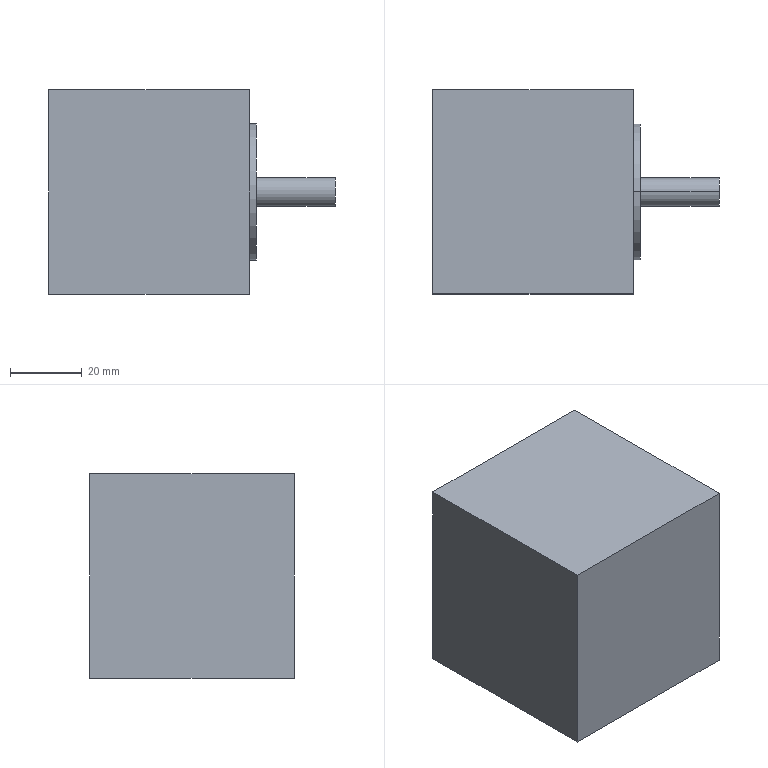Part | SolidWorks | features BaseBody 1 | 1 solid | 36 faces | box 80 x 57 x 57 mm | volume 184911 mm3 | cylinder 20 | plane 16 | commonest cylinder face diameters 3.4 x8 4.3 x8 8 x2 38 x2
STEP:
#1=CARTESIAN_POINT('',(-6.2,-23.57,25.72));
#2=VERTEX_POINT('',#1);
#3=CARTESIAN_POINT('',(-6.2,-23.57,21.42));
#4=VERTEX_POINT('',#3);
#5=CARTESIAN_POINT('',(-6.2,-23.57,23.57));
#6=DIRECTION('',(1.,0.,0.));
#7=DIRECTION('',(0.,0.,-1.));
#8=AXIS2_PLACEMENT_3D('',#5,#6,#7);
#9=CIRCLE('',#8,2.15);
#10=EDGE_CURVE('',#2,#4,#9,.T.);
#11=ORIENTED_EDGE('',*,*,#10,.F.);
#12=CARTESIAN_POINT('',(0.,-23.57,25.72));
#13=VERTEX_POINT('',#12);
#14=CARTESIAN_POINT('',(-6.2,-23.57,25.72));
#15=DIRECTION('',(1.,0.,0.));
#16=VECTOR('',#15,1000.);
#17=LINE('',#14,#16);
#18=EDGE_CURVE('',#2,#13,#17,.T.);
#19=ORIENTED_EDGE('',*,*,#18,.T.);
#20=CARTESIAN_POINT('',(0.,-23.57,21.42));
#21=VERTEX_POINT('',#20);
#22=CARTESIAN_POINT('',(0.,-23.57,23.57));
#23=DIRECTION('',(-1.,0.,0.));
#24=DIRECTION('',(0.,0.,-1.));
#25=AXIS2_PLACEMENT_3D('',#22,#23,#24);
#26=CIRCLE('',#25,2.15);
#27=EDGE_CURVE('',#21,#13,#26,.T.);
#28=ORIENTED_EDGE('',*,*,#27,.F.);
#29=CARTESIAN_POINT('',(-6.2,-23.57,21.42));
#30=DIRECTION('',(1.,0.,0.));
#31=VECTOR('',#30,1000.);
#32=LINE('',#29,#31);
#33=EDGE_CURVE('',#4,#21,#32,.T.);
#34=ORIENTED_EDGE('',*,*,#33,.F.);
#35=EDGE_LOOP('',(#11,#19,#28,#34));
#36=FACE_OUTER_BOUND('',#35,.T.);
#37=CARTESIAN_POINT('',(-6.2,-23.57,23.57));
#38=DIRECTION('',(1.,0.,0.));
#39=DIRECTION('',(0.,0.,-1.));
#40=AXIS2_PLACEMENT_3D('',#37,#38,#39);
#41=CYLINDRICAL_SURFACE('',#40,2.15);
#42=ADVANCED_FACE('',(#36),#41,.F.);
#43=CARTESIAN_POINT('',(-6.2,-23.57,-21.42));
#44=VERTEX_POINT('',#43);
#45=CARTESIAN_POINT('',(-6.2,-23.57,-25.72));
#46=VERTEX_POINT('',#45);
#47=CARTESIAN_POINT('',(-6.2,-23.57,-23.57));
#48=DIRECTION('',(1.,0.,0.));
#49=DIRECTION('',(0.,0.,-1.));
#50=AXIS2_PLACEMENT_3D('',#47,#48,#49);
#51=CIRCLE('',#50,2.15);
#52=EDGE_CURVE('',#44,#46,#51,.T.);
#53=ORIENTED_EDGE('',*,*,#52,.F.);
#54=CARTESIAN_POINT('',(0.,-23.57,-21.42));
#55=VERTEX_POINT('',#54);
#56=CARTESIAN_POINT('',(-6.2,-23.57,-21.42));
#57=DIRECTION('',(1.,0.,0.));
#58=VECTOR('',#57,1000.);
#59=LINE('',#56,#58);
#60=EDGE_CURVE('',#44,#55,#59,.T.);
#61=ORIENTED_EDGE('',*,*,#60,.T.);
#62=CARTESIAN_POINT('',(0.,-23.57,-25.72));
#63=VERTEX_POINT('',#62);
#64=CARTESIAN_POINT('',(0.,-23.57,-23.57));
#65=DIRECTION('',(-1.,0.,0.));
#66=DIRECTION('',(0.,0.,-1.));
#67=AXIS2_PLACEMENT_3D('',#64,#65,#66);
#68=CIRCLE('',#67,2.15);
#69=EDGE_CURVE('',#63,#55,#68,.T.);
#70=ORIENTED_EDGE('',*,*,#69,.F.);
#71=CARTESIAN_POINT('',(-6.2,-23.57,-25.72));
#72=DIRECTION('',(1.,0.,0.));
#73=VECTOR('',#72,1000.);
#74=LINE('',#71,#73);
#75=EDGE_CURVE('',#46,#63,#74,.T.);
#76=ORIENTED_EDGE('',*,*,#75,.F.);
#77=EDGE_LOOP('',(#53,#61,#70,#76));
#78=FACE_OUTER_BOUND('',#77,.T.);
#79=CARTESIAN_POINT('',(-6.2,-23.57,-23.57));
#80=DIRECTION('',(1.,0.,0.));
#81=DIRECTION('',(0.,0.,-1.));
#82=AXIS2_PLACEMENT_3D('',#79,#80,#81);
#83=CYLINDRICAL_SURFACE('',#82,2.15);
#84=ADVANCED_FACE('',(#78),#83,.F.);
#85=CARTESIAN_POINT('',(0.,0.,19.));
#86=VERTEX_POINT('',#85);
#87=CARTESIAN_POINT('',(0.,0.,-19.));
#88=VERTEX_POINT('',#87);
#89=CARTESIAN_POINT('',(0.,0.,0.));
#90=DIRECTION('',(-1.,0.,0.));
#91=DIRECTION('',(0.,0.,-1.));
#92=AXIS2_PLACEMENT_3D('',#89,#90,#91);
#93=CIRCLE('',#92,19.);
#94=EDGE_CURVE('',#86,#88,#93,.T.);
#95=ORIENTED_EDGE('',*,*,#94,.F.);
#96=CARTESIAN_POINT('',(2.,0.,19.));
#97=VERTEX_POINT('',#96);
#98=CARTESIAN_POINT('',(0.,0.,19.));
#99=DIRECTION('',(1.,0.,0.));
#100=VECTOR('',#99,1000.);
#101=LINE('',#98,#100);
#102=EDGE_CURVE('',#86,#97,#101,.T.);
#103=ORIENTED_EDGE('',*,*,#102,.T.);
#104=CARTESIAN_POINT('',(2.,0.,-19.));
#105=VERTEX_POINT('',#104);
#106=CARTESIAN_POINT('',(2.,0.,0.));
#107=DIRECTION('',(-1.,0.,0.));
#108=DIRECTION('',(0.,0.,-1.));
#109=AXIS2_PLACEMENT_3D('',#106,#107,#108);
#110=CIRCLE('',#109,19.);
#111=EDGE_CURVE('',#97,#105,#110,.T.);
#112=ORIENTED_EDGE('',*,*,#111,.T.);
#113=CARTESIAN_POINT('',(0.,0.,-19.));
#114=DIRECTION('',(1.,0.,0.));
#115=VECTOR('',#114,1000.);
#116=LINE('',#113,#115);
#117=EDGE_CURVE('',#88,#105,#116,.T.);
#118=ORIENTED_EDGE('',*,*,#117,.F.);
#119=EDGE_LOOP('',(#95,#103,#112,#118));
#120=FACE_OUTER_BOUND('',#119,.T.);
#121=CARTESIAN_POINT('',(0.,0.,0.));
#122=DIRECTION('',(1.,0.,0.));
#123=DIRECTION('',(0.,0.,-1.));
#124=AXIS2_PLACEMENT_3D('',#121,#122,#123);
#125=CYLINDRICAL_SURFACE('',#124,19.);
#126=ADVANCED_FACE('',(#120),#125,.T.);
#127=CARTESIAN_POINT('',(-6.2,23.57,25.72));
#128=VERTEX_POINT('',#127);
#129=CARTESIAN_POINT('',(-6.2,23.57,21.42));
#130=VERTEX_POINT('',#129);
#131=CARTESIAN_POINT('',(-6.2,23.57,23.57));
#132=DIRECTION('',(1.,0.,0.));
#133=DIRECTION('',(0.,0.,-1.));
#134=AXIS2_PLACEMENT_3D('',#131,#132,#133);
#135=CIRCLE('',#134,2.15);
#136=EDGE_CURVE('',#128,#130,#135,.T.);
#137=ORIENTED_EDGE('',*,*,#136,.F.);
#138=CARTESIAN_POINT('',(0.,23.57,25.72));
#139=VERTEX_POINT('',#138);
#140=CARTESIAN_POINT('',(-6.2,23.57,25.72));
#141=DIRECTION('',(1.,0.,0.));
#142=VECTOR('',#141,1000.);
#143=LINE('',#140,#142);
#144=EDGE_CURVE('',#128,#139,#143,.T.);
#145=ORIENTED_EDGE('',*,*,#144,.T.);
#146=CARTESIAN_POINT('',(0.,23.57,21.42));
#147=VERTEX_POINT('',#146);
#148=CARTESIAN_POINT('',(0.,23.57,23.57));
#149=DIRECTION('',(-1.,0.,0.));
#150=DIRECTION('',(0.,0.,-1.));
#151=AXIS2_PLACEMENT_3D('',#148,#149,#150);
#152=CIRCLE('',#151,2.15);
#153=EDGE_CURVE('',#147,#139,#152,.T.);
#154=ORIENTED_EDGE('',*,*,#153,.F.);
#155=CARTESIAN_POINT('',(-6.2,23.57,21.42));
#156=DIRECTION('',(1.,0.,0.));
#157=VECTOR('',#156,1000.);
#158=LINE('',#155,#157);
#159=EDGE_CURVE('',#130,#147,#158,.T.);
#160=ORIENTED_EDGE('',*,*,#159,.F.);
#161=EDGE_LOOP('',(#137,#145,#154,#160));
#162=FACE_OUTER_BOUND('',#161,.T.);
#163=CARTESIAN_POINT('',(-6.2,23.57,23.57));
#164=DIRECTION('',(1.,0.,0.));
#165=DIRECTION('',(0.,0.,-1.));
#166=AXIS2_PLACEMENT_3D('',#163,#164,#165);
#167=CYLINDRICAL_SURFACE('',#166,2.15);
#168=ADVANCED_FACE('',(#162),#167,.F.);
#169=CARTESIAN_POINT('',(-6.2,23.57,-21.42));
#170=VERTEX_POINT('',#169);
#171=CARTESIAN_POINT('',(-6.2,23.57,-25.72));
#172=VERTEX_POINT('',#171);
#173=CARTESIAN_POINT('',(-6.2,23.57,-23.57));
#174=DIRECTION('',(1.,0.,0.));
#175=DIRECTION('',(0.,0.,-1.));
#176=AXIS2_PLACEMENT_3D('',#173,#174,#175);
#177=CIRCLE('',#176,2.15);
#178=EDGE_CURVE('',#170,#172,#177,.T.);
#179=ORIENTED_EDGE('',*,*,#178,.F.);
#180=CARTESIAN_POINT('',(0.,23.57,-21.42));
#181=VERTEX_POINT('',#180);
#182=CARTESIAN_POINT('',(-6.2,23.57,-21.42));
#183=DIRECTION('',(1.,0.,0.));
#184=VECTOR('',#183,1000.);
#185=LINE('',#182,#184);
#186=EDGE_CURVE('',#170,#181,#185,.T.);
#187=ORIENTED_EDGE('',*,*,#186,.T.);
#188=CARTESIAN_POINT('',(0.,23.57,-25.72));
#189=VERTEX_POINT('',#188);
#190=CARTESIAN_POINT('',(0.,23.57,-23.57));
#191=DIRECTION('',(-1.,0.,0.));
#192=DIRECTION('',(0.,0.,-1.));
#193=AXIS2_PLACEMENT_3D('',#190,#191,#192);
#194=CIRCLE('',#193,2.15);
#195=EDGE_CURVE('',#189,#181,#194,.T.);
#196=ORIENTED_EDGE('',*,*,#195,.F.);
#197=CARTESIAN_POINT('',(-6.2,23.57,-25.72));
#198=DIRECTION('',(1.,0.,0.));
#199=VECTOR('',#198,1000.);
#200=LINE('',#197,#199);
#201=EDGE_CURVE('',#172,#189,#200,.T.);
#202=ORIENTED_EDGE('',*,*,#201,.F.);
#203=EDGE_LOOP('',(#179,#187,#196,#202));
#204=FACE_OUTER_BOUND('',#203,.T.);
#205=CARTESIAN_POINT('',(-6.2,23.57,-23.57));
#206=DIRECTION('',(1.,0.,0.));
#207=DIRECTION('',(0.,0.,-1.));
#208=AXIS2_PLACEMENT_3D('',#205,#206,#207);
#209=CYLINDRICAL_SURFACE('',#208,2.15);
#210=ADVANCED_FACE('',(#204),#209,.F.);
#211=CARTESIAN_POINT('',(-7.5,-23.57,25.27));
#212=VERTEX_POINT('',#211);
#213=CARTESIAN_POINT('',(-7.5,-23.57,21.87));
#214=VERTEX_POINT('',#213);
#215=CARTESIAN_POINT('',(-7.5,-23.57,23.57));
#216=DIRECTION('',(1.,0.,0.));
#217=DIRECTION('',(0.,0.,-1.));
#218=AXIS2_PLACEMENT_3D('',#215,#216,#217);
#219=CIRCLE('',#218,1.7);
#220=EDGE_CURVE('',#212,#214,#219,.T.);
#221=ORIENTED_EDGE('',*,*,#220,.F.);
#222=CARTESIAN_POINT('',(-6.2,-23.57,25.27));
#223=VERTEX_POINT('',#222);
#224=CARTESIAN_POINT('',(-7.5,-23.57,25.27));
#225=DIRECTION('',(1.,0.,0.));
#226=VECTOR('',#225,1000.);
#227=LINE('',#224,#226);
#228=EDGE_CURVE('',#212,#223,#227,.T.);
#229=ORIENTED_EDGE('',*,*,#228,.T.);
#230=CARTESIAN_POINT('',(-6.2,-23.57,21.87));
#231=VERTEX_POINT('',#230);
#232=CARTESIAN_POINT('',(-6.2,-23.57,23.57));
#233=DIRECTION('',(-1.,0.,0.));
#234=DIRECTION('',(0.,0.,-1.));
#235=AXIS2_PLACEMENT_3D('',#232,#233,#234);
#236=CIRCLE('',#235,1.7);
#237=EDGE_CURVE('',#231,#223,#236,.T.);
#238=ORIENTED_EDGE('',*,*,#237,.F.);
#239=CARTESIAN_POINT('',(-7.5,-23.57,21.87));
#240=DIRECTION('',(1.,0.,0.));
#241=VECTOR('',#240,1000.);
#242=LINE('',#239,#241);
#243=EDGE_CURVE('',#214,#231,#242,.T.);
#244=ORIENTED_EDGE('',*,*,#243,.F.);
#245=EDGE_LOOP('',(#221,#229,#238,#244));
#246=FACE_OUTER_BOUND('',#245,.T.);
#247=CARTESIAN_POINT('',(-7.5,-23.57,23.57));
#248=DIRECTION('',(1.,0.,0.));
#249=DIRECTION('',(0.,0.,-1.));
#250=AXIS2_PLACEMENT_3D('',#247,#248,#249);
#251=CYLINDRICAL_SURFACE('',#250,1.7);
#252=ADVANCED_FACE('',(#246),#251,.F.);
#253=CARTESIAN_POINT('',(-7.5,-23.57,-21.87));
#254=VERTEX_POINT('',#253);
#255=CARTESIAN_POINT('',(-7.5,-23.57,-25.27));
#256=VERTEX_POINT('',#255);
#257=CARTESIAN_POINT('',(-7.5,-23.57,-23.57));
#258=DIRECTION('',(1.,0.,0.));
#259=DIRECTION('',(0.,0.,-1.));
#260=AXIS2_PLACEMENT_3D('',#257,#258,#259);
#261=CIRCLE('',#260,1.7);
#262=EDGE_CURVE('',#254,#256,#261,.T.);
#263=ORIENTED_EDGE('',*,*,#262,.F.);
#264=CARTESIAN_POINT('',(-6.2,-23.57,-21.87));
#265=VERTEX_POINT('',#264);
#266=CARTESIAN_POINT('',(-7.5,-23.57,-21.87));
#267=DIRECTION('',(1.,0.,0.));
#268=VECTOR('',#267,1000.);
#269=LINE('',#266,#268);
#270=EDGE_CURVE('',#254,#265,#269,.T.);
#271=ORIENTED_EDGE('',*,*,#270,.T.);
#272=CARTESIAN_POINT('',(-6.2,-23.57,-25.27));
#273=VERTEX_POINT('',#272);
#274=CARTESIAN_POINT('',(-6.2,-23.57,-23.57));
#275=DIRECTION('',(-1.,0.,0.));
#276=DIRECTION('',(0.,0.,-1.));
#277=AXIS2_PLACEMENT_3D('',#274,#275,#276);
#278=CIRCLE('',#277,1.7);
#279=EDGE_CURVE('',#273,#265,#278,.T.);
#280=ORIENTED_EDGE('',*,*,#279,.F.);
#281=CARTESIAN_POINT('',(-7.5,-23.57,-25.27));
#282=DIRECTION('',(1.,0.,0.));
#283=VECTOR('',#282,1000.);
#284=LINE('',#281,#283);
#285=EDGE_CURVE('',#256,#273,#284,.T.);
#286=ORIENTED_EDGE('',*,*,#285,.F.);
#287=EDGE_LOOP('',(#263,#271,#280,#286));
#288=FACE_OUTER_BOUND('',#287,.T.);
#289=CARTESIAN_POINT('',(-7.5,-23.57,-23.57));
#290=DIRECTION('',(1.,0.,0.));
#291=DIRECTION('',(0.,0.,-1.));
#292=AXIS2_PLACEMENT_3D('',#289,#290,#291);
#293=CYLINDRICAL_SURFACE('',#292,1.7);
#294=ADVANCED_FACE('',(#288),#293,.F.);
#295=CARTESIAN_POINT('',(2.,0.,4.));
#296=VERTEX_POINT('',#295);
#297=CARTESIAN_POINT('',(2.,0.,-4.));
#298=VERTEX_POINT('',#297);
#299=CARTESIAN_POINT('',(2.,0.,0.));
#300=DIRECTION('',(-1.,0.,0.));
#301=DIRECTION('',(0.,0.,-1.));
#302=AXIS2_PLACEMENT_3D('',#299,#300,#301);
#303=CIRCLE('',#302,4.);
#304=EDGE_CURVE('',#296,#298,#303,.T.);
#305=ORIENTED_EDGE('',*,*,#304,.F.);
#306=CARTESIAN_POINT('',(24.,0.,4.));
#307=VERTEX_POINT('',#306);
#308=CARTESIAN_POINT('',(2.,0.,4.));
#309=DIRECTION('',(1.,0.,0.));
#310=VECTOR('',#309,1000.);
#311=LINE('',#308,#310);
#312=EDGE_CURVE('',#296,#307,#311,.T.);
#313=ORIENTED_EDGE('',*,*,#312,.T.);
#314=CARTESIAN_POINT('',(24.,0.,-4.));
#315=VERTEX_POINT('',#314);
#316=CARTESIAN_POINT('',(24.,0.,0.));
#317=DIRECTION('',(-1.,0.,0.));
#318=DIRECTION('',(0.,0.,-1.));
#319=AXIS2_PLACEMENT_3D('',#316,#317,#318);
#320=CIRCLE('',#319,4.);
#321=EDGE_CURVE('',#307,#315,#320,.T.);
#322=ORIENTED_EDGE('',*,*,#321,.T.);
#323=CARTESIAN_POINT('',(2.,0.,-4.));
#324=DIRECTION('',(1.,0.,0.));
#325=VECTOR('',#324,1000.);
#326=LINE('',#323,#325);
#327=EDGE_CURVE('',#298,#315,#326,.T.);
#328=ORIENTED_EDGE('',*,*,#327,.F.);
#329=EDGE_LOOP('',(#305,#313,#322,#328));
#330=FACE_OUTER_BOUND('',#329,.T.);
#331=CARTESIAN_POINT('',(2.,0.,0.));
#332=DIRECTION('',(1.,0.,0.));
#333=DIRECTION('',(0.,0.,-1.));
#334=AXIS2_PLACEMENT_3D('',#331,#332,#333);
#335=CYLINDRICAL_SURFACE('',#334,4.);
#336=ADVANCED_FACE('',(#330),#335,.T.);
#337=CARTESIAN_POINT('',(-7.5,23.57,25.27));
#338=VERTEX_POINT('',#337);
#339=CARTESIAN_POINT('',(-7.5,23.57,21.87));
#340=VERTEX_POINT('',#339);
#341=CARTESIAN_POINT('',(-7.5,23.57,23.57));
#342=DIRECTION('',(1.,0.,0.));
#343=DIRECTION('',(0.,0.,-1.));
#344=AXIS2_PLACEMENT_3D('',#341,#342,#343);
#345=CIRCLE('',#344,1.7);
#346=EDGE_CURVE('',#338,#340,#345,.T.);
#347=ORIENTED_EDGE('',*,*,#346,.F.);
#348=CARTESIAN_POINT('',(-6.2,23.57,25.27));
#349=VERTEX_POINT('',#348);
#350=CARTESIAN_POINT('',(-7.5,23.57,25.27));
#351=DIRECTION('',(1.,0.,0.));
#352=VECTOR('',#351,1000.);
#353=LINE('',#350,#352);
#354=EDGE_CURVE('',#338,#349,#353,.T.);
#355=ORIENTED_EDGE('',*,*,#354,.T.);
#356=CARTESIAN_POINT('',(-6.2,23.57,21.87));
#357=VERTEX_POINT('',#356);
#358=CARTESIAN_POINT('',(-6.2,23.57,23.57));
#359=DIRECTION('',(-1.,0.,0.));
#360=DIRECTION('',(0.,0.,-1.));
#361=AXIS2_PLACEMENT_3D('',#358,#359,#360);
#362=CIRCLE('',#361,1.7);
#363=EDGE_CURVE('',#357,#349,#362,.T.);
#364=ORIENTED_EDGE('',*,*,#363,.F.);
#365=CARTESIAN_POINT('',(-7.5,23.57,21.87));
#366=DIRECTION('',(1.,0.,0.));
#367=VECTOR('',#366,1000.);
#368=LINE('',#365,#367);
#369=EDGE_CURVE('',#340,#357,#368,.T.);
#370=ORIENTED_EDGE('',*,*,#369,.F.);
#371=EDGE_LOOP('',(#347,#355,#364,#370));
#372=FACE_OUTER_BOUND('',#371,.T.);
#373=CARTESIAN_POINT('',(-7.5,23.57,23.57));
#374=DIRECTION('',(1.,0.,0.));
#375=DIRECTION('',(0.,0.,-1.));
#376=AXIS2_PLACEMENT_3D('',#373,#374,#375);
#377=CYLINDRICAL_SURFACE('',#376,1.7);
#378=ADVANCED_FACE('',(#372),#377,.F.);
#379=CARTESIAN_POINT('',(-7.5,23.57,-21.87));
#380=VERTEX_POINT('',#379);
#381=CARTESIAN_POINT('',(-7.5,23.57,-25.27));
#382=VERTEX_POINT('',#381);
#383=CARTESIAN_POINT('',(-7.5,23.57,-23.57));
#384=DIRECTION('',(1.,0.,0.));
#385=DIRECTION('',(0.,0.,-1.));
#386=AXIS2_PLACEMENT_3D('',#383,#384,#385);
#387=CIRCLE('',#386,1.7);
#388=EDGE_CURVE('',#380,#382,#387,.T.);
#389=ORIENTED_EDGE('',*,*,#388,.F.);
#390=CARTESIAN_POINT('',(-6.2,23.57,-21.87));
#391=VERTEX_POINT('',#390);
#392=CARTESIAN_POINT('',(-7.5,23.57,-21.87));
#393=DIRECTION('',(1.,0.,0.));
#394=VECTOR('',#393,1000.);
#395=LINE('',#392,#394);
#396=EDGE_CURVE('',#380,#391,#395,.T.);
#397=ORIENTED_EDGE('',*,*,#396,.T.);
#398=CARTESIAN_POINT('',(-6.2,23.57,-25.27));
#399=VERTEX_POINT('',#398);
#400=CARTESIAN_POINT('',(-6.2,23.57,-23.57));
#401=DIRECTION('',(-1.,0.,0.));
#402=DIRECTION('',(0.,0.,-1.));
#403=AXIS2_PLACEMENT_3D('',#400,#401,#402);
#404=CIRCLE('',#403,1.7);
#405=EDGE_CURVE('',#399,#391,#404,.T.);
#406=ORIENTED_EDGE('',*,*,#405,.F.);
#407=CARTESIAN_POINT('',(-7.5,23.57,-25.27));
#408=DIRECTION('',(1.,0.,0.));
#409=VECTOR('',#408,1000.);
#410=LINE('',#407,#409);
#411=EDGE_CURVE('',#382,#399,#410,.T.);
#412=ORIENTED_EDGE('',*,*,#411,.F.);
#413=EDGE_LOOP('',(#389,#397,#406,#412));
#414=FACE_OUTER_BOUND('',#413,.T.);
#415=CARTESIAN_POINT('',(-7.5,23.57,-23.57));
#416=DIRECTION('',(1.,0.,0.));
#417=DIRECTION('',(0.,0.,-1.));
#418=AXIS2_PLACEMENT_3D('',#415,#416,#417);
#419=CYLINDRICAL_SURFACE('',#418,1.7);
#420=ADVANCED_FACE('',(#414),#419,.F.);
#421=CARTESIAN_POINT('',(-56.,28.5,-28.5));
#422=VERTEX_POINT('',#421);
#423=CARTESIAN_POINT('',(-56.,28.5,28.5));
#424=VERTEX_POINT('',#423);
#425=CARTESIAN_POINT('',(-56.,28.5,-28.5));
#426=DIRECTION('',(0.,0.,1.));
#427=VECTOR('',#426,1000.);
#428=LINE('',#425,#427);
#429=EDGE_CURVE('',#422,#424,#428,.T.);
#430=ORIENTED_EDGE('',*,*,#429,.F.);
#431=CARTESIAN_POINT('',(-56.,-28.5,-28.5));
#432=VERTEX_POINT('',#431);
#433=CARTESIAN_POINT('',(-56.,-28.5,-28.5));
#434=DIRECTION('',(0.,1.,0.));
#435=VECTOR('',#434,1000.);
#436=LINE('',#433,#435);
#437=EDGE_CURVE('',#432,#422,#436,.T.);
#438=ORIENTED_EDGE('',*,*,#437,.F.);
#439=CARTESIAN_POINT('',(-56.,-28.5,28.5));
#440=VERTEX_POINT('',#439);
#441=CARTESIAN_POINT('',(-56.,-28.5,-28.5));
#442=DIRECTION('',(0.,0.,-1.));
#443=VECTOR('',#442,1000.);
#444=LINE('',#441,#443);
#445=EDGE_CURVE('',#440,#432,#444,.T.);
#446=ORIENTED_EDGE('',*,*,#445,.F.);
#447=CARTESIAN_POINT('',(-56.,-28.5,28.5));
#448=DIRECTION('',(0.,-1.,0.));
#449=VECTOR('',#448,1000.);
#450=LINE('',#447,#449);
#451=EDGE_CURVE('',#424,#440,#450,.T.);
#452=ORIENTED_EDGE('',*,*,#451,.F.);
#453=EDGE_LOOP('',(#430,#438,#446,#452));
#454=FACE_OUTER_BOUND('',#453,.T.);
#455=CARTESIAN_POINT('',(-56.,-28.5,-28.5));
#456=DIRECTION('',(1.,0.,0.));
#457=DIRECTION('',(0.,0.,-1.));
#458=AXIS2_PLACEMENT_3D('',#455,#456,#457);
#459=PLANE('',#458);
#460=ADVANCED_FACE('',(#454),#459,.F.);
#461=CARTESIAN_POINT('',(0.,-28.5,28.5));
#462=VERTEX_POINT('',#461);
#463=CARTESIAN_POINT('',(0.,28.5,28.5));
#464=VERTEX_POINT('',#463);
#465=CARTESIAN_POINT('',(0.,-28.5,28.5));
#466=DIRECTION('',(0.,1.,0.));
#467=VECTOR('',#466,1000.);
#468=LINE('',#465,#467);
#469=EDGE_CURVE('',#462,#464,#468,.T.);
#470=ORIENTED_EDGE('',*,*,#469,.T.);
#471=CARTESIAN_POINT('',(-56.,28.5,28.5));
#472=DIRECTION('',(-1.,0.,0.));
#473=VECTOR('',#472,1000.);
#474=LINE('',#471,#473);
#475=EDGE_CURVE('',#464,#424,#474,.T.);
#476=ORIENTED_EDGE('',*,*,#475,.T.);
#477=ORIENTED_EDGE('',*,*,#451,.T.);
#478=CARTESIAN_POINT('',(-56.,-28.5,28.5));
#479=DIRECTION('',(1.,0.,0.));
#480=VECTOR('',#479,1000.);
#481=LINE('',#478,#480);
#482=EDGE_CURVE('',#440,#462,#481,.T.);
#483=ORIENTED_EDGE('',*,*,#482,.T.);
#484=EDGE_LOOP('',(#470,#476,#477,#483));
#485=FACE_OUTER_BOUND('',#484,.T.);
#486=CARTESIAN_POINT('',(-56.,-28.5,28.5));
#487=DIRECTION('',(0.,0.,1.));
#488=DIRECTION('',(1.,0.,0.));
#489=AXIS2_PLACEMENT_3D('',#486,#487,#488);
#490=PLANE('',#489);
#491=ADVANCED_FACE('',(#485),#490,.T.);
#492=ORIENTED_EDGE('',*,*,#475,.F.);
#493=CARTESIAN_POINT('',(0.,28.5,-28.5));
#494=VERTEX_POINT('',#493);
#495=CARTESIAN_POINT('',(0.,28.5,-28.5));
#496=DIRECTION('',(0.,0.,-1.));
#497=VECTOR('',#496,1000.);
#498=LINE('',#495,#497);
#499=EDGE_CURVE('',#464,#494,#498,.T.);
#500=ORIENTED_EDGE('',*,*,#499,.T.);
#501=CARTESIAN_POINT('',(-56.,28.5,-28.5));
#502=DIRECTION('',(-1.,0.,0.));
#503=VECTOR('',#502,1000.);
#504=LINE('',#501,#503);
#505=EDGE_CURVE('',#494,#422,#504,.T.);
#506=ORIENTED_EDGE('',*,*,#505,.T.);
#507=ORIENTED_EDGE('',*,*,#429,.T.);
#508=EDGE_LOOP('',(#492,#500,#506,#507));
#509=FACE_OUTER_BOUND('',#508,.T.);
#510=CARTESIAN_POINT('',(-56.,28.5,-28.5));
#511=DIRECTION('',(0.,1.,0.));
#512=DIRECTION('',(0.,0.,1.));
#513=AXIS2_PLACEMENT_3D('',#510,#511,#512);
#514=PLANE('',#513);
#515=ADVANCED_FACE('',(#509),#514,.T.);
#516=CARTESIAN_POINT('',(0.,-28.5,-28.5));
#517=VERTEX_POINT('',#516);
#518=CARTESIAN_POINT('',(0.,-28.5,-28.5));
#519=DIRECTION('',(0.,1.,0.));
#520=VECTOR('',#519,1000.);
#521=LINE('',#518,#520);
#522=EDGE_CURVE('',#517,#494,#521,.T.);
#523=ORIENTED_EDGE('',*,*,#522,.F.);
#524=CARTESIAN_POINT('',(-56.,-28.5,-28.5));
#525=DIRECTION('',(1.,0.,0.));
#526=VECTOR('',#525,1000.);
#527=LINE('',#524,#526);
#528=EDGE_CURVE('',#432,#517,#527,.T.);
#529=ORIENTED_EDGE('',*,*,#528,.F.);
#530=ORIENTED_EDGE('',*,*,#437,.T.);
#531=ORIENTED_EDGE('',*,*,#505,.F.);
#532=EDGE_LOOP('',(#523,#529,#530,#531));
#533=FACE_OUTER_BOUND('',#532,.T.);
#534=CARTESIAN_POINT('',(-56.,-28.5,-28.5));
#535=DIRECTION('',(0.,0.,1.));
#536=DIRECTION('',(1.,0.,0.));
#537=AXIS2_PLACEMENT_3D('',#534,#535,#536);
#538=PLANE('',#537);
#539=ADVANCED_FACE('',(#533),#538,.F.);
#540=ORIENTED_EDGE('',*,*,#482,.F.);
#541=ORIENTED_EDGE('',*,*,#445,.T.);
#542=ORIENTED_EDGE('',*,*,#528,.T.);
#543=CARTESIAN_POINT('',(0.,-28.5,-28.5));
#544=DIRECTION('',(0.,0.,-1.));
#545=VECTOR('',#544,1000.);
#546=LINE('',#543,#545);
#547=EDGE_CURVE('',#462,#517,#546,.T.);
#548=ORIENTED_EDGE('',*,*,#547,.F.);
#549=EDGE_LOOP('',(#540,#541,#542,#548));
#550=FACE_OUTER_BOUND('',#549,.T.);
#551=CARTESIAN_POINT('',(-56.,-28.5,-28.5));
#552=DIRECTION('',(0.,1.,0.));
#553=DIRECTION('',(0.,0.,1.));
#554=AXIS2_PLACEMENT_3D('',#551,#552,#553);
#555=PLANE('',#554);
#556=ADVANCED_FACE('',(#550),#555,.F.);
#557=ORIENTED_EDGE('',*,*,#27,.T.);
#558=CARTESIAN_POINT('',(0.,-23.57,23.57));
#559=DIRECTION('',(-1.,0.,0.));
#560=DIRECTION('',(0.,0.,-1.));
#561=AXIS2_PLACEMENT_3D('',#558,#559,#560);
#562=CIRCLE('',#561,2.15);
#563=EDGE_CURVE('',#13,#21,#562,.T.);
#564=ORIENTED_EDGE('',*,*,#563,.T.);
#565=EDGE_LOOP('',(#557,#564));
#566=FACE_BOUND('',#565,.T.);
#567=ORIENTED_EDGE('',*,*,#69,.T.);
#568=CARTESIAN_POINT('',(0.,-23.57,-23.57));
#569=DIRECTION('',(-1.,0.,0.));
#570=DIRECTION('',(0.,0.,-1.));
#571=AXIS2_PLACEMENT_3D('',#568,#569,#570);
#572=CIRCLE('',#571,2.15);
#573=EDGE_CURVE('',#55,#63,#572,.T.);
#574=ORIENTED_EDGE('',*,*,#573,.T.);
#575=EDGE_LOOP('',(#567,#574));
#576=FACE_BOUND('',#575,.T.);
#577=CARTESIAN_POINT('',(0.,0.,0.));
#578=DIRECTION('',(-1.,0.,0.));
#579=DIRECTION('',(0.,0.,-1.));
#580=AXIS2_PLACEMENT_3D('',#577,#578,#579);
#581=CIRCLE('',#580,19.);
#582=EDGE_CURVE('',#88,#86,#581,.T.);
#583=ORIENTED_EDGE('',*,*,#582,.T.);
#584=ORIENTED_EDGE('',*,*,#94,.T.);
#585=EDGE_LOOP('',(#583,#584));
#586=FACE_BOUND('',#585,.T.);
#587=ORIENTED_EDGE('',*,*,#153,.T.);
#588=CARTESIAN_POINT('',(0.,23.57,23.57));
#589=DIRECTION('',(-1.,0.,0.));
#590=DIRECTION('',(0.,0.,-1.));
#591=AXIS2_PLACEMENT_3D('',#588,#589,#590);
#592=CIRCLE('',#591,2.15);
#593=EDGE_CURVE('',#139,#147,#592,.T.);
#594=ORIENTED_EDGE('',*,*,#593,.T.);
#595=EDGE_LOOP('',(#587,#594));
#596=FACE_BOUND('',#595,.T.);
#597=ORIENTED_EDGE('',*,*,#195,.T.);
#598=CARTESIAN_POINT('',(0.,23.57,-23.57));
#599=DIRECTION('',(-1.,0.,0.));
#600=DIRECTION('',(0.,0.,-1.));
#601=AXIS2_PLACEMENT_3D('',#598,#599,#600);
#602=CIRCLE('',#601,2.15);
#603=EDGE_CURVE('',#181,#189,#602,.T.);
#604=ORIENTED_EDGE('',*,*,#603,.T.);
#605=EDGE_LOOP('',(#597,#604));
#606=FACE_BOUND('',#605,.T.);
#607=ORIENTED_EDGE('',*,*,#499,.F.);
#608=ORIENTED_EDGE('',*,*,#469,.F.);
#609=ORIENTED_EDGE('',*,*,#547,.T.);
#610=ORIENTED_EDGE('',*,*,#522,.T.);
#611=EDGE_LOOP('',(#607,#608,#609,#610));
#612=FACE_OUTER_BOUND('',#611,.T.);
#613=CARTESIAN_POINT('',(0.,-28.5,-28.5));
#614=DIRECTION('',(1.,0.,0.));
#615=DIRECTION('',(0.,0.,-1.));
#616=AXIS2_PLACEMENT_3D('',#613,#614,#615);
#617=PLANE('',#616);
#618=ADVANCED_FACE('',(#566,#576,#586,#596,#606,#612),#617,.T.);
#619=ORIENTED_EDGE('',*,*,#18,.F.);
#620=CARTESIAN_POINT('',(-6.2,-23.57,23.57));
#621=DIRECTION('',(1.,0.,0.));
#622=DIRECTION('',(0.,0.,-1.));
#623=AXIS2_PLACEMENT_3D('',#620,#621,#622);
#624=CIRCLE('',#623,2.15);
#625=EDGE_CURVE('',#4,#2,#624,.T.);
#626=ORIENTED_EDGE('',*,*,#625,.F.);
#627=ORIENTED_EDGE('',*,*,#33,.T.);
#628=ORIENTED_EDGE('',*,*,#563,.F.);
#629=EDGE_LOOP('',(#619,#626,#627,#628));
#630=FACE_OUTER_BOUND('',#629,.T.);
#631=CARTESIAN_POINT('',(-6.2,-23.57,23.57));
#632=DIRECTION('',(1.,0.,0.));
#633=DIRECTION('',(0.,0.,-1.));
#634=AXIS2_PLACEMENT_3D('',#631,#632,#633);
#635=CYLINDRICAL_SURFACE('',#634,2.15);
#636=ADVANCED_FACE('',(#630),#635,.F.);
#637=ORIENTED_EDGE('',*,*,#60,.F.);
#638=CARTESIAN_POINT('',(-6.2,-23.57,-23.57));
#639=DIRECTION('',(1.,0.,0.));
#640=DIRECTION('',(0.,0.,-1.));
#641=AXIS2_PLACEMENT_3D('',#638,#639,#640);
#642=CIRCLE('',#641,2.15);
#643=EDGE_CURVE('',#46,#44,#642,.T.);
#644=ORIENTED_EDGE('',*,*,#643,.F.);
#645=ORIENTED_EDGE('',*,*,#75,.T.);
#646=ORIENTED_EDGE('',*,*,#573,.F.);
#647=EDGE_LOOP('',(#637,#644,#645,#646));
#648=FACE_OUTER_BOUND('',#647,.T.);
#649=CARTESIAN_POINT('',(-6.2,-23.57,-23.57));
#650=DIRECTION('',(1.,0.,0.));
#651=DIRECTION('',(0.,0.,-1.));
#652=AXIS2_PLACEMENT_3D('',#649,#650,#651);
#653=CYLINDRICAL_SURFACE('',#652,2.15);
#654=ADVANCED_FACE('',(#648),#653,.F.);
#655=ORIENTED_EDGE('',*,*,#102,.F.);
#656=ORIENTED_EDGE('',*,*,#582,.F.);
#657=ORIENTED_EDGE('',*,*,#117,.T.);
#658=CARTESIAN_POINT('',(2.,0.,0.));
#659=DIRECTION('',(-1.,0.,0.));
#660=DIRECTION('',(0.,0.,-1.));
#661=AXIS2_PLACEMENT_3D('',#658,#659,#660);
#662=CIRCLE('',#661,19.);
#663=EDGE_CURVE('',#105,#97,#662,.T.);
#664=ORIENTED_EDGE('',*,*,#663,.T.);
#665=EDGE_LOOP('',(#655,#656,#657,#664));
#666=FACE_OUTER_BOUND('',#665,.T.);
#667=CARTESIAN_POINT('',(0.,0.,0.));
#668=DIRECTION('',(1.,0.,0.));
#669=DIRECTION('',(0.,0.,-1.));
#670=AXIS2_PLACEMENT_3D('',#667,#668,#669);
#671=CYLINDRICAL_SURFACE('',#670,19.);
#672=ADVANCED_FACE('',(#666),#671,.T.);
#673=ORIENTED_EDGE('',*,*,#144,.F.);
#674=CARTESIAN_POINT('',(-6.2,23.57,23.57));
#675=DIRECTION('',(1.,0.,0.));
#676=DIRECTION('',(0.,0.,-1.));
#677=AXIS2_PLACEMENT_3D('',#674,#675,#676);
#678=CIRCLE('',#677,2.15);
#679=EDGE_CURVE('',#130,#128,#678,.T.);
#680=ORIENTED_EDGE('',*,*,#679,.F.);
#681=ORIENTED_EDGE('',*,*,#159,.T.);
#682=ORIENTED_EDGE('',*,*,#593,.F.);
#683=EDGE_LOOP('',(#673,#680,#681,#682));
#684=FACE_OUTER_BOUND('',#683,.T.);
#685=CARTESIAN_POINT('',(-6.2,23.57,23.57));
#686=DIRECTION('',(1.,0.,0.));
#687=DIRECTION('',(0.,0.,-1.));
#688=AXIS2_PLACEMENT_3D('',#685,#686,#687);
#689=CYLINDRICAL_SURFACE('',#688,2.15);
#690=ADVANCED_FACE('',(#684),#689,.F.);
#691=ORIENTED_EDGE('',*,*,#186,.F.);
#692=CARTESIAN_POINT('',(-6.2,23.57,-23.57));
#693=DIRECTION('',(1.,0.,0.));
#694=DIRECTION('',(0.,0.,-1.));
#695=AXIS2_PLACEMENT_3D('',#692,#693,#694);
#696=CIRCLE('',#695,2.15);
#697=EDGE_CURVE('',#172,#170,#696,.T.);
#698=ORIENTED_EDGE('',*,*,#697,.F.);
#699=ORIENTED_EDGE('',*,*,#201,.T.);
#700=ORIENTED_EDGE('',*,*,#603,.F.);
#701=EDGE_LOOP('',(#691,#698,#699,#700));
#702=FACE_OUTER_BOUND('',#701,.T.);
#703=CARTESIAN_POINT('',(-6.2,23.57,-23.57));
#704=DIRECTION('',(1.,0.,0.));
#705=DIRECTION('',(0.,0.,-1.));
#706=AXIS2_PLACEMENT_3D('',#703,#704,#705);
#707=CYLINDRICAL_SURFACE('',#706,2.15);
#708=ADVANCED_FACE('',(#702),#707,.F.);
#709=ORIENTED_EDGE('',*,*,#237,.T.);
#710=CARTESIAN_POINT('',(-6.2,-23.57,23.57));
#711=DIRECTION('',(-1.,0.,0.));
#712=DIRECTION('',(0.,0.,-1.));
#713=AXIS2_PLACEMENT_3D('',#710,#711,#712);
#714=CIRCLE('',#713,1.7);
#715=EDGE_CURVE('',#223,#231,#714,.T.);
#716=ORIENTED_EDGE('',*,*,#715,.T.);
#717=EDGE_LOOP('',(#709,#716));
#718=FACE_BOUND('',#717,.T.);
#719=ORIENTED_EDGE('',*,*,#625,.T.);
#720=ORIENTED_EDGE('',*,*,#10,.T.);
#721=EDGE_LOOP('',(#719,#720));
#722=FACE_OUTER_BOUND('',#721,.T.);
#723=CARTESIAN_POINT('',(-6.2,-23.57,23.57));
#724=DIRECTION('',(1.,0.,0.));
#725=DIRECTION('',(0.,0.,-1.));
#726=AXIS2_PLACEMENT_3D('',#723,#724,#725);
#727=PLANE('',#726);
#728=ADVANCED_FACE('',(#718,#722),#727,.T.);
#729=ORIENTED_EDGE('',*,*,#279,.T.);
#730=CARTESIAN_POINT('',(-6.2,-23.57,-23.57));
#731=DIRECTION('',(-1.,0.,0.));
#732=DIRECTION('',(0.,0.,-1.));
#733=AXIS2_PLACEMENT_3D('',#730,#731,#732);
#734=CIRCLE('',#733,1.7);
#735=EDGE_CURVE('',#265,#273,#734,.T.);
#736=ORIENTED_EDGE('',*,*,#735,.T.);
#737=EDGE_LOOP('',(#729,#736));
#738=FACE_BOUND('',#737,.T.);
#739=ORIENTED_EDGE('',*,*,#643,.T.);
#740=ORIENTED_EDGE('',*,*,#52,.T.);
#741=EDGE_LOOP('',(#739,#740));
#742=FACE_OUTER_BOUND('',#741,.T.);
#743=CARTESIAN_POINT('',(-6.2,-23.57,-23.57));
#744=DIRECTION('',(1.,0.,0.));
#745=DIRECTION('',(0.,0.,-1.));
#746=AXIS2_PLACEMENT_3D('',#743,#744,#745);
#747=PLANE('',#746);
#748=ADVANCED_FACE('',(#738,#742),#747,.T.);
#749=CARTESIAN_POINT('',(2.,0.,0.));
#750=DIRECTION('',(-1.,0.,0.));
#751=DIRECTION('',(0.,0.,-1.));
#752=AXIS2_PLACEMENT_3D('',#749,#750,#751);
#753=CIRCLE('',#752,4.);
#754=EDGE_CURVE('',#298,#296,#753,.T.);
#755=ORIENTED_EDGE('',*,*,#754,.T.);
#756=ORIENTED_EDGE('',*,*,#304,.T.);
#757=EDGE_LOOP('',(#755,#756));
#758=FACE_BOUND('',#757,.T.);
#759=ORIENTED_EDGE('',*,*,#663,.F.);
#760=ORIENTED_EDGE('',*,*,#111,.F.);
#761=EDGE_LOOP('',(#759,#760));
#762=FACE_OUTER_BOUND('',#761,.T.);
#763=CARTESIAN_POINT('',(2.,0.,0.));
#764=DIRECTION('',(1.,0.,0.));
#765=DIRECTION('',(0.,0.,-1.));
#766=AXIS2_PLACEMENT_3D('',#763,#764,#765);
#767=PLANE('',#766);
#768=ADVANCED_FACE('',(#758,#762),#767,.T.);
#769=ORIENTED_EDGE('',*,*,#363,.T.);
#770=CARTESIAN_POINT('',(-6.2,23.57,23.57));
#771=DIRECTION('',(-1.,0.,0.));
#772=DIRECTION('',(0.,0.,-1.));
#773=AXIS2_PLACEMENT_3D('',#770,#771,#772);
#774=CIRCLE('',#773,1.7);
#775=EDGE_CURVE('',#349,#357,#774,.T.);
#776=ORIENTED_EDGE('',*,*,#775,.T.);
#777=EDGE_LOOP('',(#769,#776));
#778=FACE_BOUND('',#777,.T.);
#779=ORIENTED_EDGE('',*,*,#679,.T.);
#780=ORIENTED_EDGE('',*,*,#136,.T.);
#781=EDGE_LOOP('',(#779,#780));
#782=FACE_OUTER_BOUND('',#781,.T.);
#783=CARTESIAN_POINT('',(-6.2,23.57,23.57));
#784=DIRECTION('',(1.,0.,0.));
#785=DIRECTION('',(0.,0.,-1.));
#786=AXIS2_PLACEMENT_3D('',#783,#784,#785);
#787=PLANE('',#786);
#788=ADVANCED_FACE('',(#778,#782),#787,.T.);
#789=ORIENTED_EDGE('',*,*,#405,.T.);
#790=CARTESIAN_POINT('',(-6.2,23.57,-23.57));
#791=DIRECTION('',(-1.,0.,0.));
#792=DIRECTION('',(0.,0.,-1.));
#793=AXIS2_PLACEMENT_3D('',#790,#791,#792);
#794=CIRCLE('',#793,1.7);
#795=EDGE_CURVE('',#391,#399,#794,.T.);
#796=ORIENTED_EDGE('',*,*,#795,.T.);
#797=EDGE_LOOP('',(#789,#796));
#798=FACE_BOUND('',#797,.T.);
#799=ORIENTED_EDGE('',*,*,#697,.T.);
#800=ORIENTED_EDGE('',*,*,#178,.T.);
#801=EDGE_LOOP('',(#799,#800));
#802=FACE_OUTER_BOUND('',#801,.T.);
#803=CARTESIAN_POINT('',(-6.2,23.57,-23.57));
#804=DIRECTION('',(1.,0.,0.));
#805=DIRECTION('',(0.,0.,-1.));
#806=AXIS2_PLACEMENT_3D('',#803,#804,#805);
#807=PLANE('',#806);
#808=ADVANCED_FACE('',(#798,#802),#807,.T.);
#809=ORIENTED_EDGE('',*,*,#228,.F.);
#810=CARTESIAN_POINT('',(-7.5,-23.57,23.57));
#811=DIRECTION('',(1.,0.,0.));
#812=DIRECTION('',(0.,0.,-1.));
#813=AXIS2_PLACEMENT_3D('',#810,#811,#812);
#814=CIRCLE('',#813,1.7);
#815=EDGE_CURVE('',#214,#212,#814,.T.);
#816=ORIENTED_EDGE('',*,*,#815,.F.);
#817=ORIENTED_EDGE('',*,*,#243,.T.);
#818=ORIENTED_EDGE('',*,*,#715,.F.);
#819=EDGE_LOOP('',(#809,#816,#817,#818));
#820=FACE_OUTER_BOUND('',#819,.T.);
#821=CARTESIAN_POINT('',(-7.5,-23.57,23.57));
#822=DIRECTION('',(1.,0.,0.));
#823=DIRECTION('',(0.,0.,-1.));
#824=AXIS2_PLACEMENT_3D('',#821,#822,#823);
#825=CYLINDRICAL_SURFACE('',#824,1.7);
#826=ADVANCED_FACE('',(#820),#825,.F.);
#827=ORIENTED_EDGE('',*,*,#270,.F.);
#828=CARTESIAN_POINT('',(-7.5,-23.57,-23.57));
#829=DIRECTION('',(1.,0.,0.));
#830=DIRECTION('',(0.,0.,-1.));
#831=AXIS2_PLACEMENT_3D('',#828,#829,#830);
#832=CIRCLE('',#831,1.7);
#833=EDGE_CURVE('',#256,#254,#832,.T.);
#834=ORIENTED_EDGE('',*,*,#833,.F.);
#835=ORIENTED_EDGE('',*,*,#285,.T.);
#836=ORIENTED_EDGE('',*,*,#735,.F.);
#837=EDGE_LOOP('',(#827,#834,#835,#836));
#838=FACE_OUTER_BOUND('',#837,.T.);
#839=CARTESIAN_POINT('',(-7.5,-23.57,-23.57));
#840=DIRECTION('',(1.,0.,0.));
#841=DIRECTION('',(0.,0.,-1.));
#842=AXIS2_PLACEMENT_3D('',#839,#840,#841);
#843=CYLINDRICAL_SURFACE('',#842,1.7);
#844=ADVANCED_FACE('',(#838),#843,.F.);
#845=ORIENTED_EDGE('',*,*,#312,.F.);
#846=ORIENTED_EDGE('',*,*,#754,.F.);
#847=ORIENTED_EDGE('',*,*,#327,.T.);
#848=CARTESIAN_POINT('',(24.,0.,0.));
#849=DIRECTION('',(-1.,0.,0.));
#850=DIRECTION('',(0.,0.,-1.));
#851=AXIS2_PLACEMENT_3D('',#848,#849,#850);
#852=CIRCLE('',#851,4.);
#853=EDGE_CURVE('',#315,#307,#852,.T.);
#854=ORIENTED_EDGE('',*,*,#853,.T.);
#855=EDGE_LOOP('',(#845,#846,#847,#854));
#856=FACE_OUTER_BOUND('',#855,.T.);
#857=CARTESIAN_POINT('',(2.,0.,0.));
#858=DIRECTION('',(1.,0.,0.));
#859=DIRECTION('',(0.,0.,-1.));
#860=AXIS2_PLACEMENT_3D('',#857,#858,#859);
#861=CYLINDRICAL_SURFACE('',#860,4.);
#862=ADVANCED_FACE('',(#856),#861,.T.);
#863=ORIENTED_EDGE('',*,*,#354,.F.);
#864=CARTESIAN_POINT('',(-7.5,23.57,23.57));
#865=DIRECTION('',(1.,0.,0.));
#866=DIRECTION('',(0.,0.,-1.));
#867=AXIS2_PLACEMENT_3D('',#864,#865,#866);
#868=CIRCLE('',#867,1.7);
#869=EDGE_CURVE('',#340,#338,#868,.T.);
#870=ORIENTED_EDGE('',*,*,#869,.F.);
#871=ORIENTED_EDGE('',*,*,#369,.T.);
#872=ORIENTED_EDGE('',*,*,#775,.F.);
#873=EDGE_LOOP('',(#863,#870,#871,#872));
#874=FACE_OUTER_BOUND('',#873,.T.);
#875=CARTESIAN_POINT('',(-7.5,23.57,23.57));
#876=DIRECTION('',(1.,0.,0.));
#877=DIRECTION('',(0.,0.,-1.));
#878=AXIS2_PLACEMENT_3D('',#875,#876,#877);
#879=CYLINDRICAL_SURFACE('',#878,1.7);
#880=ADVANCED_FACE('',(#874),#879,.F.);
#881=ORIENTED_EDGE('',*,*,#396,.F.);
#882=CARTESIAN_POINT('',(-7.5,23.57,-23.57));
#883=DIRECTION('',(1.,0.,0.));
#884=DIRECTION('',(0.,0.,-1.));
#885=AXIS2_PLACEMENT_3D('',#882,#883,#884);
#886=CIRCLE('',#885,1.7);
#887=EDGE_CURVE('',#382,#380,#886,.T.);
#888=ORIENTED_EDGE('',*,*,#887,.F.);
#889=ORIENTED_EDGE('',*,*,#411,.T.);
#890=ORIENTED_EDGE('',*,*,#795,.F.);
#891=EDGE_LOOP('',(#881,#888,#889,#890));
#892=FACE_OUTER_BOUND('',#891,.T.);
#893=CARTESIAN_POINT('',(-7.5,23.57,-23.57));
#894=DIRECTION('',(1.,0.,0.));
#895=DIRECTION('',(0.,0.,-1.));
#896=AXIS2_PLACEMENT_3D('',#893,#894,#895);
#897=CYLINDRICAL_SURFACE('',#896,1.7);
#898=ADVANCED_FACE('',(#892),#897,.F.);
#899=ORIENTED_EDGE('',*,*,#815,.T.);
#900=ORIENTED_EDGE('',*,*,#220,.T.);
#901=EDGE_LOOP('',(#899,#900));
#902=FACE_OUTER_BOUND('',#901,.T.);
#903=CARTESIAN_POINT('',(-7.5,-23.57,23.57));
#904=DIRECTION('',(1.,0.,0.));
#905=DIRECTION('',(0.,0.,-1.));
#906=AXIS2_PLACEMENT_3D('',#903,#904,#905);
#907=PLANE('',#906);
#908=ADVANCED_FACE('',(#902),#907,.T.);
#909=ORIENTED_EDGE('',*,*,#833,.T.);
#910=ORIENTED_EDGE('',*,*,#262,.T.);
#911=EDGE_LOOP('',(#909,#910));
#912=FACE_OUTER_BOUND('',#911,.T.);
#913=CARTESIAN_POINT('',(-7.5,-23.57,-23.57));
#914=DIRECTION('',(1.,0.,0.));
#915=DIRECTION('',(0.,0.,-1.));
#916=AXIS2_PLACEMENT_3D('',#913,#914,#915);
#917=PLANE('',#916);
#918=ADVANCED_FACE('',(#912),#917,.T.);
#919=ORIENTED_EDGE('',*,*,#853,.F.);
#920=ORIENTED_EDGE('',*,*,#321,.F.);
#921=EDGE_LOOP('',(#919,#920));
#922=FACE_OUTER_BOUND('',#921,.T.);
#923=CARTESIAN_POINT('',(24.,0.,0.));
#924=DIRECTION('',(1.,0.,0.));
#925=DIRECTION('',(0.,0.,-1.));
#926=AXIS2_PLACEMENT_3D('',#923,#924,#925);
#927=PLANE('',#926);
#928=ADVANCED_FACE('',(#922),#927,.T.);
#929=ORIENTED_EDGE('',*,*,#869,.T.);
#930=ORIENTED_EDGE('',*,*,#346,.T.);
#931=EDGE_LOOP('',(#929,#930));
#932=FACE_OUTER_BOUND('',#931,.T.);
#933=CARTESIAN_POINT('',(-7.5,23.57,23.57));
#934=DIRECTION('',(1.,0.,0.));
#935=DIRECTION('',(0.,0.,-1.));
#936=AXIS2_PLACEMENT_3D('',#933,#934,#935);
#937=PLANE('',#936);
#938=ADVANCED_FACE('',(#932),#937,.T.);
#939=ORIENTED_EDGE('',*,*,#887,.T.);
#940=ORIENTED_EDGE('',*,*,#388,.T.);
#941=EDGE_LOOP('',(#939,#940));
#942=FACE_OUTER_BOUND('',#941,.T.);
#943=CARTESIAN_POINT('',(-7.5,23.57,-23.57));
#944=DIRECTION('',(1.,0.,0.));
#945=DIRECTION('',(0.,0.,-1.));
#946=AXIS2_PLACEMENT_3D('',#943,#944,#945);
#947=PLANE('',#946);
#948=ADVANCED_FACE('',(#942),#947,.T.);
#949=CLOSED_SHELL('',(#42,#84,#126,#168,#210,#252,#294,#336,#378,#420,#460,#491,#515,#539,#556,#618,#636,#654,#672,#690,#708,#728,#748,#768,#788,#808,#826,#844,#862,#880,#898,#908,#918,#928,#938,#948));
#950=MANIFOLD_SOLID_BREP('',#949);
#951=CARTESIAN_POINT('',(0.,0.,0.));
#952=DIRECTION('',(0.,0.,1.));
#953=DIRECTION('',(1.,0.,0.));
#954=AXIS2_PLACEMENT_3D('',#951,#952,#953);
#955=(LENGTH_UNIT()NAMED_UNIT(*)SI_UNIT(.MILLI.,.METRE.));
#956=UNCERTAINTY_MEASURE_WITH_UNIT(LENGTH_MEASURE(0.00001),#955,'','');
#957=(NAMED_UNIT(*)PLANE_ANGLE_UNIT()SI_UNIT($,.RADIAN.));
#958=(NAMED_UNIT(*)SI_UNIT($,.STERADIAN.)SOLID_ANGLE_UNIT());
#959=(GEOMETRIC_REPRESENTATION_CONTEXT(3)GLOBAL_UNCERTAINTY_ASSIGNED_CONTEXT((#956))GLOBAL_UNIT_ASSIGNED_CONTEXT((#955,#957,#958))REPRESENTATION_CONTEXT('',''));
#960=ADVANCED_BREP_SHAPE_REPRESENTATION('',(#950,#954),#959);